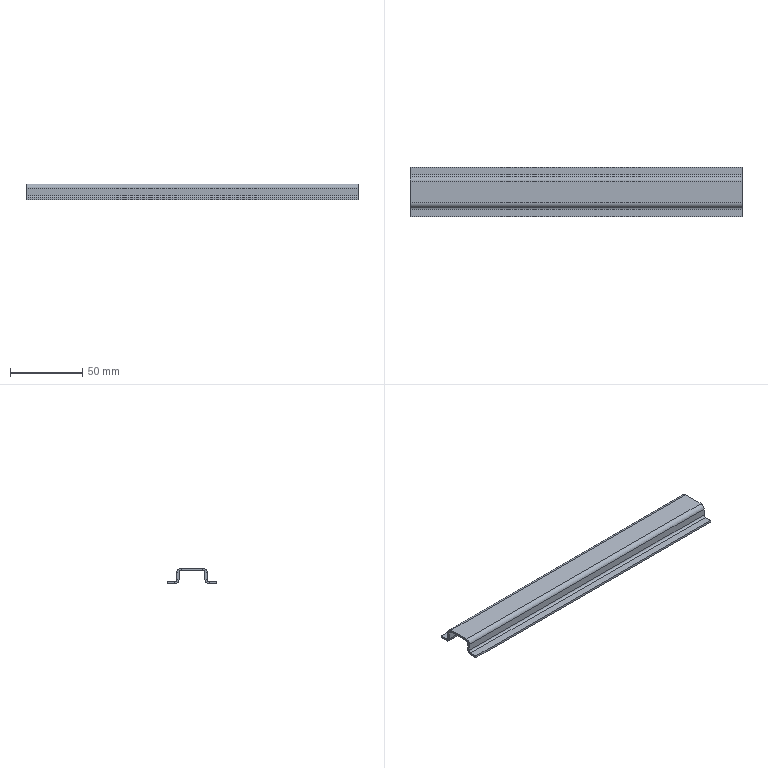Part | SolidWorks | features EdgeFlange 2, FlatPattern 1, SMBaseFlange 1, SheetMetal 1 | 1 solid | 38 faces | box 230 x 34 x 11 mm | volume 16952 mm3 | plane 30 | cylinder 8 | commonest cylinder face diameters 3 x4 6 x4
STEP:
#1=CARTESIAN_POINT('',(115.,-7.5,0.));
#2=VERTEX_POINT('',#1);
#3=CARTESIAN_POINT('',(115.,7.5,0.));
#4=VERTEX_POINT('',#3);
#5=CARTESIAN_POINT('',(115.,-7.5,0.));
#6=DIRECTION('',(0.,1.,0.));
#7=VECTOR('',#6,1000.);
#8=LINE('',#5,#7);
#9=EDGE_CURVE('',#2,#4,#8,.T.);
#10=ORIENTED_EDGE('',*,*,#9,.F.);
#11=CARTESIAN_POINT('',(115.,-7.5,-1.5));
#12=VERTEX_POINT('',#11);
#13=CARTESIAN_POINT('',(115.,-7.5,-1.5));
#14=DIRECTION('',(0.,0.,1.));
#15=VECTOR('',#14,1000.);
#16=LINE('',#13,#15);
#17=EDGE_CURVE('',#12,#2,#16,.T.);
#18=ORIENTED_EDGE('',*,*,#17,.F.);
#19=CARTESIAN_POINT('',(115.,7.5,-1.5));
#20=VERTEX_POINT('',#19);
#21=CARTESIAN_POINT('',(115.,-7.5,-1.5));
#22=DIRECTION('',(0.,1.,0.));
#23=VECTOR('',#22,1000.);
#24=LINE('',#21,#23);
#25=EDGE_CURVE('',#12,#20,#24,.T.);
#26=ORIENTED_EDGE('',*,*,#25,.T.);
#27=CARTESIAN_POINT('',(115.,7.5,-1.5));
#28=DIRECTION('',(0.,0.,1.));
#29=VECTOR('',#28,1000.);
#30=LINE('',#27,#29);
#31=EDGE_CURVE('',#20,#4,#30,.T.);
#32=ORIENTED_EDGE('',*,*,#31,.T.);
#33=EDGE_LOOP('',(#10,#18,#26,#32));
#34=FACE_OUTER_BOUND('',#33,.T.);
#35=CARTESIAN_POINT('',(115.,-7.5,-1.5));
#36=DIRECTION('',(1.,0.,0.));
#37=DIRECTION('',(0.,0.,-1.));
#38=AXIS2_PLACEMENT_3D('',#35,#36,#37);
#39=PLANE('',#38);
#40=ADVANCED_FACE('',(#34),#39,.T.);
#41=CARTESIAN_POINT('',(-115.,7.5,0.));
#42=VERTEX_POINT('',#41);
#43=CARTESIAN_POINT('',(-115.,-7.5,0.));
#44=VERTEX_POINT('',#43);
#45=CARTESIAN_POINT('',(-115.,-7.5,0.));
#46=DIRECTION('',(0.,-1.,0.));
#47=VECTOR('',#46,1000.);
#48=LINE('',#45,#47);
#49=EDGE_CURVE('',#42,#44,#48,.T.);
#50=ORIENTED_EDGE('',*,*,#49,.F.);
#51=CARTESIAN_POINT('',(-115.,7.5,-1.5));
#52=VERTEX_POINT('',#51);
#53=CARTESIAN_POINT('',(-115.,7.5,-1.5));
#54=DIRECTION('',(0.,0.,1.));
#55=VECTOR('',#54,1000.);
#56=LINE('',#53,#55);
#57=EDGE_CURVE('',#52,#42,#56,.T.);
#58=ORIENTED_EDGE('',*,*,#57,.F.);
#59=CARTESIAN_POINT('',(-115.,-7.5,-1.5));
#60=VERTEX_POINT('',#59);
#61=CARTESIAN_POINT('',(-115.,-7.5,-1.5));
#62=DIRECTION('',(0.,-1.,0.));
#63=VECTOR('',#62,1000.);
#64=LINE('',#61,#63);
#65=EDGE_CURVE('',#52,#60,#64,.T.);
#66=ORIENTED_EDGE('',*,*,#65,.T.);
#67=CARTESIAN_POINT('',(-115.,-7.5,-1.5));
#68=DIRECTION('',(0.,0.,1.));
#69=VECTOR('',#68,1000.);
#70=LINE('',#67,#69);
#71=EDGE_CURVE('',#60,#44,#70,.T.);
#72=ORIENTED_EDGE('',*,*,#71,.T.);
#73=EDGE_LOOP('',(#50,#58,#66,#72));
#74=FACE_OUTER_BOUND('',#73,.T.);
#75=CARTESIAN_POINT('',(-115.,-7.5,-1.5));
#76=DIRECTION('',(-1.,0.,0.));
#77=DIRECTION('',(0.,0.,1.));
#78=AXIS2_PLACEMENT_3D('',#75,#76,#77);
#79=PLANE('',#78);
#80=ADVANCED_FACE('',(#74),#79,.T.);
#81=ORIENTED_EDGE('',*,*,#25,.F.);
#82=CARTESIAN_POINT('',(-115.,-7.5,-1.5));
#83=DIRECTION('',(1.,0.,0.));
#84=VECTOR('',#83,1000.);
#85=LINE('',#82,#84);
#86=EDGE_CURVE('',#60,#12,#85,.T.);
#87=ORIENTED_EDGE('',*,*,#86,.F.);
#88=ORIENTED_EDGE('',*,*,#65,.F.);
#89=CARTESIAN_POINT('',(-115.,7.5,-1.5));
#90=DIRECTION('',(-1.,0.,0.));
#91=VECTOR('',#90,1000.);
#92=LINE('',#89,#91);
#93=EDGE_CURVE('',#20,#52,#92,.T.);
#94=ORIENTED_EDGE('',*,*,#93,.F.);
#95=EDGE_LOOP('',(#81,#87,#88,#94));
#96=FACE_OUTER_BOUND('',#95,.T.);
#97=CARTESIAN_POINT('',(0.,0.,-1.5));
#98=DIRECTION('',(0.,0.,-1.));
#99=DIRECTION('',(-1.,0.,0.));
#100=AXIS2_PLACEMENT_3D('',#97,#98,#99);
#101=PLANE('',#100);
#102=ADVANCED_FACE('',(#96),#101,.T.);
#103=ORIENTED_EDGE('',*,*,#9,.T.);
#104=CARTESIAN_POINT('',(-115.,7.5,0.));
#105=DIRECTION('',(-1.,0.,0.));
#106=VECTOR('',#105,1000.);
#107=LINE('',#104,#106);
#108=EDGE_CURVE('',#4,#42,#107,.T.);
#109=ORIENTED_EDGE('',*,*,#108,.T.);
#110=ORIENTED_EDGE('',*,*,#49,.T.);
#111=CARTESIAN_POINT('',(-115.,-7.5,0.));
#112=DIRECTION('',(1.,0.,0.));
#113=VECTOR('',#112,1000.);
#114=LINE('',#111,#113);
#115=EDGE_CURVE('',#44,#2,#114,.T.);
#116=ORIENTED_EDGE('',*,*,#115,.T.);
#117=EDGE_LOOP('',(#103,#109,#110,#116));
#118=FACE_OUTER_BOUND('',#117,.T.);
#119=CARTESIAN_POINT('',(0.,0.,0.));
#120=DIRECTION('',(0.,0.,-1.));
#121=DIRECTION('',(-1.,0.,0.));
#122=AXIS2_PLACEMENT_3D('',#119,#120,#121);
#123=PLANE('',#122);
#124=ADVANCED_FACE('',(#118),#123,.F.);
#125=CARTESIAN_POINT('',(-115.,9.,-3.));
#126=VERTEX_POINT('',#125);
#127=CARTESIAN_POINT('',(-115.,10.5,-3.));
#128=VERTEX_POINT('',#127);
#129=CARTESIAN_POINT('',(-115.,10.5,-3.));
#130=DIRECTION('',(0.,1.,0.));
#131=VECTOR('',#130,1000.);
#132=LINE('',#129,#131);
#133=EDGE_CURVE('',#126,#128,#132,.T.);
#134=ORIENTED_EDGE('',*,*,#133,.F.);
#135=CARTESIAN_POINT('',(-115.,7.5,-3.));
#136=DIRECTION('',(-1.,0.,0.));
#137=DIRECTION('',(0.,0.,-1.));
#138=AXIS2_PLACEMENT_3D('',#135,#136,#137);
#139=CIRCLE('',#138,1.5);
#140=EDGE_CURVE('',#52,#126,#139,.T.);
#141=ORIENTED_EDGE('',*,*,#140,.F.);
#142=ORIENTED_EDGE('',*,*,#57,.T.);
#143=CARTESIAN_POINT('',(-115.,7.5,-3.));
#144=DIRECTION('',(-1.,0.,0.));
#145=DIRECTION('',(0.,0.,-1.));
#146=AXIS2_PLACEMENT_3D('',#143,#144,#145);
#147=CIRCLE('',#146,3.);
#148=EDGE_CURVE('',#42,#128,#147,.T.);
#149=ORIENTED_EDGE('',*,*,#148,.T.);
#150=EDGE_LOOP('',(#134,#141,#142,#149));
#151=FACE_OUTER_BOUND('',#150,.T.);
#152=CARTESIAN_POINT('',(-115.,7.5,-3.));
#153=DIRECTION('',(-1.,0.,0.));
#154=DIRECTION('',(0.,0.,1.));
#155=AXIS2_PLACEMENT_3D('',#152,#153,#154);
#156=PLANE('',#155);
#157=ADVANCED_FACE('',(#151),#156,.T.);
#158=CARTESIAN_POINT('',(115.,9.,-3.));
#159=VERTEX_POINT('',#158);
#160=CARTESIAN_POINT('',(115.,7.5,-3.));
#161=DIRECTION('',(1.,0.,0.));
#162=DIRECTION('',(0.,0.,-1.));
#163=AXIS2_PLACEMENT_3D('',#160,#161,#162);
#164=CIRCLE('',#163,1.5);
#165=EDGE_CURVE('',#159,#20,#164,.T.);
#166=ORIENTED_EDGE('',*,*,#165,.F.);
#167=CARTESIAN_POINT('',(115.,10.5,-3.));
#168=VERTEX_POINT('',#167);
#169=CARTESIAN_POINT('',(115.,9.,-3.));
#170=DIRECTION('',(0.,1.,0.));
#171=VECTOR('',#170,1000.);
#172=LINE('',#169,#171);
#173=EDGE_CURVE('',#159,#168,#172,.T.);
#174=ORIENTED_EDGE('',*,*,#173,.T.);
#175=CARTESIAN_POINT('',(115.,7.5,-3.));
#176=DIRECTION('',(1.,0.,0.));
#177=DIRECTION('',(0.,0.,-1.));
#178=AXIS2_PLACEMENT_3D('',#175,#176,#177);
#179=CIRCLE('',#178,3.);
#180=EDGE_CURVE('',#168,#4,#179,.T.);
#181=ORIENTED_EDGE('',*,*,#180,.T.);
#182=ORIENTED_EDGE('',*,*,#31,.F.);
#183=EDGE_LOOP('',(#166,#174,#181,#182));
#184=FACE_OUTER_BOUND('',#183,.T.);
#185=CARTESIAN_POINT('',(115.,7.5,-3.));
#186=DIRECTION('',(-1.,0.,0.));
#187=DIRECTION('',(0.,0.,1.));
#188=AXIS2_PLACEMENT_3D('',#185,#186,#187);
#189=PLANE('',#188);
#190=ADVANCED_FACE('',(#184),#189,.F.);
#191=ORIENTED_EDGE('',*,*,#108,.F.);
#192=ORIENTED_EDGE('',*,*,#180,.F.);
#193=CARTESIAN_POINT('',(-115.,10.5,-3.));
#194=DIRECTION('',(-1.,0.,0.));
#195=VECTOR('',#194,1000.);
#196=LINE('',#193,#195);
#197=EDGE_CURVE('',#168,#128,#196,.T.);
#198=ORIENTED_EDGE('',*,*,#197,.T.);
#199=ORIENTED_EDGE('',*,*,#148,.F.);
#200=EDGE_LOOP('',(#191,#192,#198,#199));
#201=FACE_OUTER_BOUND('',#200,.T.);
#202=CARTESIAN_POINT('',(115.,7.5,-3.));
#203=DIRECTION('',(1.,0.,0.));
#204=DIRECTION('',(0.,1.,0.));
#205=AXIS2_PLACEMENT_3D('',#202,#203,#204);
#206=CYLINDRICAL_SURFACE('',#205,3.);
#207=ADVANCED_FACE('',(#201),#206,.T.);
#208=ORIENTED_EDGE('',*,*,#93,.T.);
#209=ORIENTED_EDGE('',*,*,#140,.T.);
#210=CARTESIAN_POINT('',(-115.,9.,-3.));
#211=DIRECTION('',(1.,0.,0.));
#212=VECTOR('',#211,1000.);
#213=LINE('',#210,#212);
#214=EDGE_CURVE('',#126,#159,#213,.T.);
#215=ORIENTED_EDGE('',*,*,#214,.T.);
#216=ORIENTED_EDGE('',*,*,#165,.T.);
#217=EDGE_LOOP('',(#208,#209,#215,#216));
#218=FACE_OUTER_BOUND('',#217,.T.);
#219=CARTESIAN_POINT('',(115.,7.5,-3.));
#220=DIRECTION('',(1.,0.,0.));
#221=DIRECTION('',(0.,1.,0.));
#222=AXIS2_PLACEMENT_3D('',#219,#220,#221);
#223=CYLINDRICAL_SURFACE('',#222,1.5);
#224=ADVANCED_FACE('',(#218),#223,.F.);
#225=ORIENTED_EDGE('',*,*,#173,.F.);
#226=CARTESIAN_POINT('',(115.,9.,-8.));
#227=VERTEX_POINT('',#226);
#228=CARTESIAN_POINT('',(115.,9.,-8.));
#229=DIRECTION('',(0.,0.,-1.));
#230=VECTOR('',#229,1000.);
#231=LINE('',#228,#230);
#232=EDGE_CURVE('',#159,#227,#231,.T.);
#233=ORIENTED_EDGE('',*,*,#232,.T.);
#234=CARTESIAN_POINT('',(115.,10.5,-8.));
#235=VERTEX_POINT('',#234);
#236=CARTESIAN_POINT('',(115.,10.5,-8.));
#237=DIRECTION('',(0.,-1.,0.));
#238=VECTOR('',#237,1000.);
#239=LINE('',#236,#238);
#240=EDGE_CURVE('',#235,#227,#239,.T.);
#241=ORIENTED_EDGE('',*,*,#240,.F.);
#242=CARTESIAN_POINT('',(115.,10.5,0.));
#243=DIRECTION('',(0.,0.,-1.));
#244=VECTOR('',#243,1000.);
#245=LINE('',#242,#244);
#246=EDGE_CURVE('',#168,#235,#245,.T.);
#247=ORIENTED_EDGE('',*,*,#246,.F.);
#248=EDGE_LOOP('',(#225,#233,#241,#247));
#249=FACE_OUTER_BOUND('',#248,.T.);
#250=CARTESIAN_POINT('',(115.,10.5,-8.));
#251=DIRECTION('',(-1.,0.,0.));
#252=DIRECTION('',(0.,0.,1.));
#253=AXIS2_PLACEMENT_3D('',#250,#251,#252);
#254=PLANE('',#253);
#255=ADVANCED_FACE('',(#249),#254,.F.);
#256=ORIENTED_EDGE('',*,*,#133,.T.);
#257=CARTESIAN_POINT('',(-115.,10.5,-8.));
#258=VERTEX_POINT('',#257);
#259=CARTESIAN_POINT('',(-115.,10.5,0.));
#260=DIRECTION('',(0.,0.,1.));
#261=VECTOR('',#260,1000.);
#262=LINE('',#259,#261);
#263=EDGE_CURVE('',#258,#128,#262,.T.);
#264=ORIENTED_EDGE('',*,*,#263,.F.);
#265=CARTESIAN_POINT('',(-115.,9.,-8.));
#266=VERTEX_POINT('',#265);
#267=CARTESIAN_POINT('',(-115.,10.5,-8.));
#268=DIRECTION('',(0.,-1.,0.));
#269=VECTOR('',#268,1000.);
#270=LINE('',#267,#269);
#271=EDGE_CURVE('',#258,#266,#270,.T.);
#272=ORIENTED_EDGE('',*,*,#271,.T.);
#273=CARTESIAN_POINT('',(-115.,9.,-1.5));
#274=DIRECTION('',(0.,0.,1.));
#275=VECTOR('',#274,1000.);
#276=LINE('',#273,#275);
#277=EDGE_CURVE('',#266,#126,#276,.T.);
#278=ORIENTED_EDGE('',*,*,#277,.T.);
#279=EDGE_LOOP('',(#256,#264,#272,#278));
#280=FACE_OUTER_BOUND('',#279,.T.);
#281=CARTESIAN_POINT('',(-115.,10.5,-1.5));
#282=DIRECTION('',(1.,0.,0.));
#283=DIRECTION('',(0.,0.,-1.));
#284=AXIS2_PLACEMENT_3D('',#281,#282,#283);
#285=PLANE('',#284);
#286=ADVANCED_FACE('',(#280),#285,.F.);
#287=ORIENTED_EDGE('',*,*,#197,.F.);
#288=ORIENTED_EDGE('',*,*,#246,.T.);
#289=CARTESIAN_POINT('',(0.,10.5,-8.));
#290=DIRECTION('',(-1.,0.,0.));
#291=VECTOR('',#290,1000.);
#292=LINE('',#289,#291);
#293=EDGE_CURVE('',#235,#258,#292,.T.);
#294=ORIENTED_EDGE('',*,*,#293,.T.);
#295=ORIENTED_EDGE('',*,*,#263,.T.);
#296=EDGE_LOOP('',(#287,#288,#294,#295));
#297=FACE_OUTER_BOUND('',#296,.T.);
#298=CARTESIAN_POINT('',(0.,10.5,0.));
#299=DIRECTION('',(0.,-1.,0.));
#300=DIRECTION('',(0.,0.,-1.));
#301=AXIS2_PLACEMENT_3D('',#298,#299,#300);
#302=PLANE('',#301);
#303=ADVANCED_FACE('',(#297),#302,.F.);
#304=ORIENTED_EDGE('',*,*,#232,.F.);
#305=ORIENTED_EDGE('',*,*,#214,.F.);
#306=ORIENTED_EDGE('',*,*,#277,.F.);
#307=CARTESIAN_POINT('',(-115.,9.,-8.));
#308=DIRECTION('',(-1.,0.,0.));
#309=VECTOR('',#308,1000.);
#310=LINE('',#307,#309);
#311=EDGE_CURVE('',#227,#266,#310,.T.);
#312=ORIENTED_EDGE('',*,*,#311,.F.);
#313=EDGE_LOOP('',(#304,#305,#306,#312));
#314=FACE_OUTER_BOUND('',#313,.T.);
#315=CARTESIAN_POINT('',(0.,9.,0.));
#316=DIRECTION('',(0.,-1.,0.));
#317=DIRECTION('',(0.,0.,-1.));
#318=AXIS2_PLACEMENT_3D('',#315,#316,#317);
#319=PLANE('',#318);
#320=ADVANCED_FACE('',(#314),#319,.T.);
#321=CARTESIAN_POINT('',(115.,-9.,-3.));
#322=VERTEX_POINT('',#321);
#323=CARTESIAN_POINT('',(115.,-10.5,-3.));
#324=VERTEX_POINT('',#323);
#325=CARTESIAN_POINT('',(115.,-10.5,-3.));
#326=DIRECTION('',(0.,-1.,0.));
#327=VECTOR('',#326,1000.);
#328=LINE('',#325,#327);
#329=EDGE_CURVE('',#322,#324,#328,.T.);
#330=ORIENTED_EDGE('',*,*,#329,.F.);
#331=CARTESIAN_POINT('',(115.,-7.5,-3.));
#332=DIRECTION('',(1.,0.,0.));
#333=DIRECTION('',(0.,0.,1.));
#334=AXIS2_PLACEMENT_3D('',#331,#332,#333);
#335=CIRCLE('',#334,1.5);
#336=EDGE_CURVE('',#12,#322,#335,.T.);
#337=ORIENTED_EDGE('',*,*,#336,.F.);
#338=ORIENTED_EDGE('',*,*,#17,.T.);
#339=CARTESIAN_POINT('',(115.,-7.5,-3.));
#340=DIRECTION('',(1.,0.,0.));
#341=DIRECTION('',(0.,0.,1.));
#342=AXIS2_PLACEMENT_3D('',#339,#340,#341);
#343=CIRCLE('',#342,3.);
#344=EDGE_CURVE('',#2,#324,#343,.T.);
#345=ORIENTED_EDGE('',*,*,#344,.T.);
#346=EDGE_LOOP('',(#330,#337,#338,#345));
#347=FACE_OUTER_BOUND('',#346,.T.);
#348=CARTESIAN_POINT('',(115.,-7.5,-3.));
#349=DIRECTION('',(1.,0.,0.));
#350=DIRECTION('',(0.,0.,-1.));
#351=AXIS2_PLACEMENT_3D('',#348,#349,#350);
#352=PLANE('',#351);
#353=ADVANCED_FACE('',(#347),#352,.T.);
#354=CARTESIAN_POINT('',(-115.,-9.,-3.));
#355=VERTEX_POINT('',#354);
#356=CARTESIAN_POINT('',(-115.,-7.5,-3.));
#357=DIRECTION('',(-1.,0.,0.));
#358=DIRECTION('',(0.,0.,1.));
#359=AXIS2_PLACEMENT_3D('',#356,#357,#358);
#360=CIRCLE('',#359,1.5);
#361=EDGE_CURVE('',#355,#60,#360,.T.);
#362=ORIENTED_EDGE('',*,*,#361,.F.);
#363=CARTESIAN_POINT('',(-115.,-10.5,-3.));
#364=VERTEX_POINT('',#363);
#365=CARTESIAN_POINT('',(-115.,-9.,-3.));
#366=DIRECTION('',(0.,-1.,0.));
#367=VECTOR('',#366,1000.);
#368=LINE('',#365,#367);
#369=EDGE_CURVE('',#355,#364,#368,.T.);
#370=ORIENTED_EDGE('',*,*,#369,.T.);
#371=CARTESIAN_POINT('',(-115.,-7.5,-3.));
#372=DIRECTION('',(-1.,0.,0.));
#373=DIRECTION('',(0.,0.,1.));
#374=AXIS2_PLACEMENT_3D('',#371,#372,#373);
#375=CIRCLE('',#374,3.);
#376=EDGE_CURVE('',#364,#44,#375,.T.);
#377=ORIENTED_EDGE('',*,*,#376,.T.);
#378=ORIENTED_EDGE('',*,*,#71,.F.);
#379=EDGE_LOOP('',(#362,#370,#377,#378));
#380=FACE_OUTER_BOUND('',#379,.T.);
#381=CARTESIAN_POINT('',(-115.,-7.5,-3.));
#382=DIRECTION('',(1.,0.,0.));
#383=DIRECTION('',(0.,0.,-1.));
#384=AXIS2_PLACEMENT_3D('',#381,#382,#383);
#385=PLANE('',#384);
#386=ADVANCED_FACE('',(#380),#385,.F.);
#387=ORIENTED_EDGE('',*,*,#115,.F.);
#388=ORIENTED_EDGE('',*,*,#376,.F.);
#389=CARTESIAN_POINT('',(115.,-10.5,-3.));
#390=DIRECTION('',(1.,0.,0.));
#391=VECTOR('',#390,1000.);
#392=LINE('',#389,#391);
#393=EDGE_CURVE('',#364,#324,#392,.T.);
#394=ORIENTED_EDGE('',*,*,#393,.T.);
#395=ORIENTED_EDGE('',*,*,#344,.F.);
#396=EDGE_LOOP('',(#387,#388,#394,#395));
#397=FACE_OUTER_BOUND('',#396,.T.);
#398=CARTESIAN_POINT('',(-115.,-7.5,-3.));
#399=DIRECTION('',(-1.,0.,0.));
#400=DIRECTION('',(0.,-1.,0.));
#401=AXIS2_PLACEMENT_3D('',#398,#399,#400);
#402=CYLINDRICAL_SURFACE('',#401,3.);
#403=ADVANCED_FACE('',(#397),#402,.T.);
#404=ORIENTED_EDGE('',*,*,#86,.T.);
#405=ORIENTED_EDGE('',*,*,#336,.T.);
#406=CARTESIAN_POINT('',(115.,-9.,-3.));
#407=DIRECTION('',(-1.,0.,0.));
#408=VECTOR('',#407,1000.);
#409=LINE('',#406,#408);
#410=EDGE_CURVE('',#322,#355,#409,.T.);
#411=ORIENTED_EDGE('',*,*,#410,.T.);
#412=ORIENTED_EDGE('',*,*,#361,.T.);
#413=EDGE_LOOP('',(#404,#405,#411,#412));
#414=FACE_OUTER_BOUND('',#413,.T.);
#415=CARTESIAN_POINT('',(-115.,-7.5,-3.));
#416=DIRECTION('',(-1.,0.,0.));
#417=DIRECTION('',(0.,-1.,0.));
#418=AXIS2_PLACEMENT_3D('',#415,#416,#417);
#419=CYLINDRICAL_SURFACE('',#418,1.5);
#420=ADVANCED_FACE('',(#414),#419,.F.);
#421=ORIENTED_EDGE('',*,*,#369,.F.);
#422=CARTESIAN_POINT('',(-115.,-9.,-8.));
#423=VERTEX_POINT('',#422);
#424=CARTESIAN_POINT('',(-115.,-9.,-8.));
#425=DIRECTION('',(0.,0.,-1.));
#426=VECTOR('',#425,1000.);
#427=LINE('',#424,#426);
#428=EDGE_CURVE('',#355,#423,#427,.T.);
#429=ORIENTED_EDGE('',*,*,#428,.T.);
#430=CARTESIAN_POINT('',(-115.,-10.5,-8.));
#431=VERTEX_POINT('',#430);
#432=CARTESIAN_POINT('',(-115.,-10.5,-8.));
#433=DIRECTION('',(0.,1.,0.));
#434=VECTOR('',#433,1000.);
#435=LINE('',#432,#434);
#436=EDGE_CURVE('',#431,#423,#435,.T.);
#437=ORIENTED_EDGE('',*,*,#436,.F.);
#438=CARTESIAN_POINT('',(-115.,-10.5,0.));
#439=DIRECTION('',(0.,0.,-1.));
#440=VECTOR('',#439,1000.);
#441=LINE('',#438,#440);
#442=EDGE_CURVE('',#364,#431,#441,.T.);
#443=ORIENTED_EDGE('',*,*,#442,.F.);
#444=EDGE_LOOP('',(#421,#429,#437,#443));
#445=FACE_OUTER_BOUND('',#444,.T.);
#446=CARTESIAN_POINT('',(-115.,-10.5,-8.));
#447=DIRECTION('',(1.,0.,0.));
#448=DIRECTION('',(0.,0.,-1.));
#449=AXIS2_PLACEMENT_3D('',#446,#447,#448);
#450=PLANE('',#449);
#451=ADVANCED_FACE('',(#445),#450,.F.);
#452=ORIENTED_EDGE('',*,*,#329,.T.);
#453=CARTESIAN_POINT('',(115.,-10.5,-8.));
#454=VERTEX_POINT('',#453);
#455=CARTESIAN_POINT('',(115.,-10.5,0.));
#456=DIRECTION('',(0.,0.,1.));
#457=VECTOR('',#456,1000.);
#458=LINE('',#455,#457);
#459=EDGE_CURVE('',#454,#324,#458,.T.);
#460=ORIENTED_EDGE('',*,*,#459,.F.);
#461=CARTESIAN_POINT('',(115.,-9.,-8.));
#462=VERTEX_POINT('',#461);
#463=CARTESIAN_POINT('',(115.,-10.5,-8.));
#464=DIRECTION('',(0.,1.,0.));
#465=VECTOR('',#464,1000.);
#466=LINE('',#463,#465);
#467=EDGE_CURVE('',#454,#462,#466,.T.);
#468=ORIENTED_EDGE('',*,*,#467,.T.);
#469=CARTESIAN_POINT('',(115.,-9.,-1.5));
#470=DIRECTION('',(0.,0.,1.));
#471=VECTOR('',#470,1000.);
#472=LINE('',#469,#471);
#473=EDGE_CURVE('',#462,#322,#472,.T.);
#474=ORIENTED_EDGE('',*,*,#473,.T.);
#475=EDGE_LOOP('',(#452,#460,#468,#474));
#476=FACE_OUTER_BOUND('',#475,.T.);
#477=CARTESIAN_POINT('',(115.,-10.5,-1.5));
#478=DIRECTION('',(-1.,0.,0.));
#479=DIRECTION('',(0.,0.,1.));
#480=AXIS2_PLACEMENT_3D('',#477,#478,#479);
#481=PLANE('',#480);
#482=ADVANCED_FACE('',(#476),#481,.F.);
#483=ORIENTED_EDGE('',*,*,#393,.F.);
#484=ORIENTED_EDGE('',*,*,#442,.T.);
#485=CARTESIAN_POINT('',(0.,-10.5,-8.));
#486=DIRECTION('',(1.,0.,0.));
#487=VECTOR('',#486,1000.);
#488=LINE('',#485,#487);
#489=EDGE_CURVE('',#431,#454,#488,.T.);
#490=ORIENTED_EDGE('',*,*,#489,.T.);
#491=ORIENTED_EDGE('',*,*,#459,.T.);
#492=EDGE_LOOP('',(#483,#484,#490,#491));
#493=FACE_OUTER_BOUND('',#492,.T.);
#494=CARTESIAN_POINT('',(0.,-10.5,0.));
#495=DIRECTION('',(0.,1.,0.));
#496=DIRECTION('',(0.,0.,1.));
#497=AXIS2_PLACEMENT_3D('',#494,#495,#496);
#498=PLANE('',#497);
#499=ADVANCED_FACE('',(#493),#498,.F.);
#500=ORIENTED_EDGE('',*,*,#428,.F.);
#501=ORIENTED_EDGE('',*,*,#410,.F.);
#502=ORIENTED_EDGE('',*,*,#473,.F.);
#503=CARTESIAN_POINT('',(115.,-9.,-8.));
#504=DIRECTION('',(1.,0.,0.));
#505=VECTOR('',#504,1000.);
#506=LINE('',#503,#505);
#507=EDGE_CURVE('',#423,#462,#506,.T.);
#508=ORIENTED_EDGE('',*,*,#507,.F.);
#509=EDGE_LOOP('',(#500,#501,#502,#508));
#510=FACE_OUTER_BOUND('',#509,.T.);
#511=CARTESIAN_POINT('',(0.,-9.,0.));
#512=DIRECTION('',(0.,1.,0.));
#513=DIRECTION('',(0.,0.,1.));
#514=AXIS2_PLACEMENT_3D('',#511,#512,#513);
#515=PLANE('',#514);
#516=ADVANCED_FACE('',(#510),#515,.T.);
#517=CARTESIAN_POINT('',(115.,12.,-9.5));
#518=VERTEX_POINT('',#517);
#519=CARTESIAN_POINT('',(115.,12.,-11.));
#520=VERTEX_POINT('',#519);
#521=CARTESIAN_POINT('',(115.,12.,-11.));
#522=DIRECTION('',(0.,0.,-1.));
#523=VECTOR('',#522,1000.);
#524=LINE('',#521,#523);
#525=EDGE_CURVE('',#518,#520,#524,.T.);
#526=ORIENTED_EDGE('',*,*,#525,.F.);
#527=CARTESIAN_POINT('',(115.,12.,-8.));
#528=DIRECTION('',(1.,0.,0.));
#529=DIRECTION('',(0.,0.,1.));
#530=AXIS2_PLACEMENT_3D('',#527,#528,#529);
#531=CIRCLE('',#530,1.5);
#532=EDGE_CURVE('',#235,#518,#531,.T.);
#533=ORIENTED_EDGE('',*,*,#532,.F.);
#534=ORIENTED_EDGE('',*,*,#240,.T.);
#535=CARTESIAN_POINT('',(115.,12.,-8.));
#536=DIRECTION('',(1.,0.,0.));
#537=DIRECTION('',(0.,0.,1.));
#538=AXIS2_PLACEMENT_3D('',#535,#536,#537);
#539=CIRCLE('',#538,3.);
#540=EDGE_CURVE('',#227,#520,#539,.T.);
#541=ORIENTED_EDGE('',*,*,#540,.T.);
#542=EDGE_LOOP('',(#526,#533,#534,#541));
#543=FACE_OUTER_BOUND('',#542,.T.);
#544=CARTESIAN_POINT('',(115.,12.,-8.));
#545=DIRECTION('',(1.,0.,0.));
#546=DIRECTION('',(0.,0.,-1.));
#547=AXIS2_PLACEMENT_3D('',#544,#545,#546);
#548=PLANE('',#547);
#549=ADVANCED_FACE('',(#543),#548,.T.);
#550=CARTESIAN_POINT('',(-115.,12.,-9.5));
#551=VERTEX_POINT('',#550);
#552=CARTESIAN_POINT('',(-115.,12.,-8.));
#553=DIRECTION('',(-1.,0.,0.));
#554=DIRECTION('',(0.,0.,1.));
#555=AXIS2_PLACEMENT_3D('',#552,#553,#554);
#556=CIRCLE('',#555,1.5);
#557=EDGE_CURVE('',#551,#258,#556,.T.);
#558=ORIENTED_EDGE('',*,*,#557,.F.);
#559=CARTESIAN_POINT('',(-115.,12.,-11.));
#560=VERTEX_POINT('',#559);
#561=CARTESIAN_POINT('',(-115.,12.,-9.5));
#562=DIRECTION('',(0.,0.,-1.));
#563=VECTOR('',#562,1000.);
#564=LINE('',#561,#563);
#565=EDGE_CURVE('',#551,#560,#564,.T.);
#566=ORIENTED_EDGE('',*,*,#565,.T.);
#567=CARTESIAN_POINT('',(-115.,12.,-8.));
#568=DIRECTION('',(-1.,0.,0.));
#569=DIRECTION('',(0.,0.,1.));
#570=AXIS2_PLACEMENT_3D('',#567,#568,#569);
#571=CIRCLE('',#570,3.);
#572=EDGE_CURVE('',#560,#266,#571,.T.);
#573=ORIENTED_EDGE('',*,*,#572,.T.);
#574=ORIENTED_EDGE('',*,*,#271,.F.);
#575=EDGE_LOOP('',(#558,#566,#573,#574));
#576=FACE_OUTER_BOUND('',#575,.T.);
#577=CARTESIAN_POINT('',(-115.,12.,-8.));
#578=DIRECTION('',(1.,0.,0.));
#579=DIRECTION('',(0.,0.,-1.));
#580=AXIS2_PLACEMENT_3D('',#577,#578,#579);
#581=PLANE('',#580);
#582=ADVANCED_FACE('',(#576),#581,.F.);
#583=ORIENTED_EDGE('',*,*,#311,.T.);
#584=ORIENTED_EDGE('',*,*,#572,.F.);
#585=CARTESIAN_POINT('',(0.,12.,-11.));
#586=DIRECTION('',(-1.,0.,0.));
#587=VECTOR('',#586,1000.);
#588=LINE('',#585,#587);
#589=EDGE_CURVE('',#520,#560,#588,.T.);
#590=ORIENTED_EDGE('',*,*,#589,.F.);
#591=ORIENTED_EDGE('',*,*,#540,.F.);
#592=EDGE_LOOP('',(#583,#584,#590,#591));
#593=FACE_OUTER_BOUND('',#592,.T.);
#594=CARTESIAN_POINT('',(-115.,12.,-8.));
#595=DIRECTION('',(-1.,0.,0.));
#596=DIRECTION('',(0.,0.,-1.));
#597=AXIS2_PLACEMENT_3D('',#594,#595,#596);
#598=CYLINDRICAL_SURFACE('',#597,3.);
#599=ADVANCED_FACE('',(#593),#598,.T.);
#600=ORIENTED_EDGE('',*,*,#293,.F.);
#601=ORIENTED_EDGE('',*,*,#532,.T.);
#602=CARTESIAN_POINT('',(115.,12.,-9.5));
#603=DIRECTION('',(-1.,0.,0.));
#604=VECTOR('',#603,1000.);
#605=LINE('',#602,#604);
#606=EDGE_CURVE('',#518,#551,#605,.T.);
#607=ORIENTED_EDGE('',*,*,#606,.T.);
#608=ORIENTED_EDGE('',*,*,#557,.T.);
#609=EDGE_LOOP('',(#600,#601,#607,#608));
#610=FACE_OUTER_BOUND('',#609,.T.);
#611=CARTESIAN_POINT('',(-115.,12.,-8.));
#612=DIRECTION('',(-1.,0.,0.));
#613=DIRECTION('',(0.,0.,-1.));
#614=AXIS2_PLACEMENT_3D('',#611,#612,#613);
#615=CYLINDRICAL_SURFACE('',#614,1.5);
#616=ADVANCED_FACE('',(#610),#615,.F.);
#617=CARTESIAN_POINT('',(-115.,17.,-11.));
#618=VERTEX_POINT('',#617);
#619=CARTESIAN_POINT('',(-115.,10.5,-11.));
#620=DIRECTION('',(0.,-1.,0.));
#621=VECTOR('',#620,1000.);
#622=LINE('',#619,#621);
#623=EDGE_CURVE('',#618,#560,#622,.T.);
#624=ORIENTED_EDGE('',*,*,#623,.T.);
#625=ORIENTED_EDGE('',*,*,#565,.F.);
#626=CARTESIAN_POINT('',(-115.,17.,-9.5));
#627=VERTEX_POINT('',#626);
#628=CARTESIAN_POINT('',(-115.,0.,-9.5));
#629=DIRECTION('',(0.,-1.,0.));
#630=VECTOR('',#629,1000.);
#631=LINE('',#628,#630);
#632=EDGE_CURVE('',#627,#551,#631,.T.);
#633=ORIENTED_EDGE('',*,*,#632,.F.);
#634=CARTESIAN_POINT('',(-115.,17.,-11.));
#635=DIRECTION('',(0.,0.,1.));
#636=VECTOR('',#635,1000.);
#637=LINE('',#634,#636);
#638=EDGE_CURVE('',#618,#627,#637,.T.);
#639=ORIENTED_EDGE('',*,*,#638,.F.);
#640=EDGE_LOOP('',(#624,#625,#633,#639));
#641=FACE_OUTER_BOUND('',#640,.T.);
#642=CARTESIAN_POINT('',(-115.,10.5,-11.));
#643=DIRECTION('',(-1.,0.,0.));
#644=DIRECTION('',(0.,0.,1.));
#645=AXIS2_PLACEMENT_3D('',#642,#643,#644);
#646=PLANE('',#645);
#647=ADVANCED_FACE('',(#641),#646,.T.);
#648=CARTESIAN_POINT('',(115.,17.,-9.5));
#649=VERTEX_POINT('',#648);
#650=CARTESIAN_POINT('',(115.,0.,-9.5));
#651=DIRECTION('',(0.,1.,0.));
#652=VECTOR('',#651,1000.);
#653=LINE('',#650,#652);
#654=EDGE_CURVE('',#518,#649,#653,.T.);
#655=ORIENTED_EDGE('',*,*,#654,.F.);
#656=ORIENTED_EDGE('',*,*,#525,.T.);
#657=CARTESIAN_POINT('',(115.,17.,-11.));
#658=VERTEX_POINT('',#657);
#659=CARTESIAN_POINT('',(115.,17.,-11.));
#660=DIRECTION('',(0.,1.,0.));
#661=VECTOR('',#660,1000.);
#662=LINE('',#659,#661);
#663=EDGE_CURVE('',#520,#658,#662,.T.);
#664=ORIENTED_EDGE('',*,*,#663,.T.);
#665=CARTESIAN_POINT('',(115.,17.,-11.));
#666=DIRECTION('',(0.,0.,1.));
#667=VECTOR('',#666,1000.);
#668=LINE('',#665,#667);
#669=EDGE_CURVE('',#658,#649,#668,.T.);
#670=ORIENTED_EDGE('',*,*,#669,.T.);
#671=EDGE_LOOP('',(#655,#656,#664,#670));
#672=FACE_OUTER_BOUND('',#671,.T.);
#673=CARTESIAN_POINT('',(115.,17.,-11.));
#674=DIRECTION('',(1.,0.,0.));
#675=DIRECTION('',(0.,0.,-1.));
#676=AXIS2_PLACEMENT_3D('',#673,#674,#675);
#677=PLANE('',#676);
#678=ADVANCED_FACE('',(#672),#677,.T.);
#679=ORIENTED_EDGE('',*,*,#663,.F.);
#680=ORIENTED_EDGE('',*,*,#589,.T.);
#681=ORIENTED_EDGE('',*,*,#623,.F.);
#682=CARTESIAN_POINT('',(-115.,17.,-11.));
#683=DIRECTION('',(-1.,0.,0.));
#684=VECTOR('',#683,1000.);
#685=LINE('',#682,#684);
#686=EDGE_CURVE('',#658,#618,#685,.T.);
#687=ORIENTED_EDGE('',*,*,#686,.F.);
#688=EDGE_LOOP('',(#679,#680,#681,#687));
#689=FACE_OUTER_BOUND('',#688,.T.);
#690=CARTESIAN_POINT('',(0.,0.,-11.));
#691=DIRECTION('',(0.,0.,-1.));
#692=DIRECTION('',(-1.,0.,0.));
#693=AXIS2_PLACEMENT_3D('',#690,#691,#692);
#694=PLANE('',#693);
#695=ADVANCED_FACE('',(#689),#694,.T.);
#696=ORIENTED_EDGE('',*,*,#606,.F.);
#697=ORIENTED_EDGE('',*,*,#654,.T.);
#698=CARTESIAN_POINT('',(0.,17.,-9.5));
#699=DIRECTION('',(-1.,0.,0.));
#700=VECTOR('',#699,1000.);
#701=LINE('',#698,#700);
#702=EDGE_CURVE('',#649,#627,#701,.T.);
#703=ORIENTED_EDGE('',*,*,#702,.T.);
#704=ORIENTED_EDGE('',*,*,#632,.T.);
#705=EDGE_LOOP('',(#696,#697,#703,#704));
#706=FACE_OUTER_BOUND('',#705,.T.);
#707=CARTESIAN_POINT('',(0.,0.,-9.5));
#708=DIRECTION('',(0.,0.,-1.));
#709=DIRECTION('',(-1.,0.,0.));
#710=AXIS2_PLACEMENT_3D('',#707,#708,#709);
#711=PLANE('',#710);
#712=ADVANCED_FACE('',(#706),#711,.F.);
#713=ORIENTED_EDGE('',*,*,#702,.F.);
#714=ORIENTED_EDGE('',*,*,#669,.F.);
#715=ORIENTED_EDGE('',*,*,#686,.T.);
#716=ORIENTED_EDGE('',*,*,#638,.T.);
#717=EDGE_LOOP('',(#713,#714,#715,#716));
#718=FACE_OUTER_BOUND('',#717,.T.);
#719=CARTESIAN_POINT('',(-115.,17.,-11.));
#720=DIRECTION('',(0.,1.,0.));
#721=DIRECTION('',(0.,0.,1.));
#722=AXIS2_PLACEMENT_3D('',#719,#720,#721);
#723=PLANE('',#722);
#724=ADVANCED_FACE('',(#718),#723,.T.);
#725=CARTESIAN_POINT('',(-115.,-12.,-9.5));
#726=VERTEX_POINT('',#725);
#727=CARTESIAN_POINT('',(-115.,-12.,-11.));
#728=VERTEX_POINT('',#727);
#729=CARTESIAN_POINT('',(-115.,-12.,-11.));
#730=DIRECTION('',(0.,0.,-1.));
#731=VECTOR('',#730,1000.);
#732=LINE('',#729,#731);
#733=EDGE_CURVE('',#726,#728,#732,.T.);
#734=ORIENTED_EDGE('',*,*,#733,.F.);
#735=CARTESIAN_POINT('',(-115.,-12.,-8.));
#736=DIRECTION('',(-1.,0.,0.));
#737=DIRECTION('',(0.,0.,-1.));
#738=AXIS2_PLACEMENT_3D('',#735,#736,#737);
#739=CIRCLE('',#738,1.5);
#740=EDGE_CURVE('',#431,#726,#739,.T.);
#741=ORIENTED_EDGE('',*,*,#740,.F.);
#742=ORIENTED_EDGE('',*,*,#436,.T.);
#743=CARTESIAN_POINT('',(-115.,-12.,-8.));
#744=DIRECTION('',(-1.,0.,0.));
#745=DIRECTION('',(0.,0.,-1.));
#746=AXIS2_PLACEMENT_3D('',#743,#744,#745);
#747=CIRCLE('',#746,3.);
#748=EDGE_CURVE('',#423,#728,#747,.T.);
#749=ORIENTED_EDGE('',*,*,#748,.T.);
#750=EDGE_LOOP('',(#734,#741,#742,#749));
#751=FACE_OUTER_BOUND('',#750,.T.);
#752=CARTESIAN_POINT('',(-115.,-12.,-8.));
#753=DIRECTION('',(-1.,0.,0.));
#754=DIRECTION('',(0.,0.,1.));
#755=AXIS2_PLACEMENT_3D('',#752,#753,#754);
#756=PLANE('',#755);
#757=ADVANCED_FACE('',(#751),#756,.T.);
#758=CARTESIAN_POINT('',(115.,-12.,-9.5));
#759=VERTEX_POINT('',#758);
#760=CARTESIAN_POINT('',(115.,-12.,-8.));
#761=DIRECTION('',(1.,0.,0.));
#762=DIRECTION('',(0.,0.,-1.));
#763=AXIS2_PLACEMENT_3D('',#760,#761,#762);
#764=CIRCLE('',#763,1.5);
#765=EDGE_CURVE('',#759,#454,#764,.T.);
#766=ORIENTED_EDGE('',*,*,#765,.F.);
#767=CARTESIAN_POINT('',(115.,-12.,-11.));
#768=VERTEX_POINT('',#767);
#769=CARTESIAN_POINT('',(115.,-12.,-9.5));
#770=DIRECTION('',(0.,0.,-1.));
#771=VECTOR('',#770,1000.);
#772=LINE('',#769,#771);
#773=EDGE_CURVE('',#759,#768,#772,.T.);
#774=ORIENTED_EDGE('',*,*,#773,.T.);
#775=CARTESIAN_POINT('',(115.,-12.,-8.));
#776=DIRECTION('',(1.,0.,0.));
#777=DIRECTION('',(0.,0.,-1.));
#778=AXIS2_PLACEMENT_3D('',#775,#776,#777);
#779=CIRCLE('',#778,3.);
#780=EDGE_CURVE('',#768,#462,#779,.T.);
#781=ORIENTED_EDGE('',*,*,#780,.T.);
#782=ORIENTED_EDGE('',*,*,#467,.F.);
#783=EDGE_LOOP('',(#766,#774,#781,#782));
#784=FACE_OUTER_BOUND('',#783,.T.);
#785=CARTESIAN_POINT('',(115.,-12.,-8.));
#786=DIRECTION('',(-1.,0.,0.));
#787=DIRECTION('',(0.,0.,1.));
#788=AXIS2_PLACEMENT_3D('',#785,#786,#787);
#789=PLANE('',#788);
#790=ADVANCED_FACE('',(#784),#789,.F.);
#791=ORIENTED_EDGE('',*,*,#507,.T.);
#792=ORIENTED_EDGE('',*,*,#780,.F.);
#793=CARTESIAN_POINT('',(-115.,-12.,-11.));
#794=DIRECTION('',(-1.,0.,0.));
#795=VECTOR('',#794,1000.);
#796=LINE('',#793,#795);
#797=EDGE_CURVE('',#768,#728,#796,.T.);
#798=ORIENTED_EDGE('',*,*,#797,.T.);
#799=ORIENTED_EDGE('',*,*,#748,.F.);
#800=EDGE_LOOP('',(#791,#792,#798,#799));
#801=FACE_OUTER_BOUND('',#800,.T.);
#802=CARTESIAN_POINT('',(115.,-12.,-8.));
#803=DIRECTION('',(1.,0.,0.));
#804=DIRECTION('',(0.,0.,-1.));
#805=AXIS2_PLACEMENT_3D('',#802,#803,#804);
#806=CYLINDRICAL_SURFACE('',#805,3.);
#807=ADVANCED_FACE('',(#801),#806,.T.);
#808=ORIENTED_EDGE('',*,*,#489,.F.);
#809=ORIENTED_EDGE('',*,*,#740,.T.);
#810=CARTESIAN_POINT('',(-115.,-12.,-9.5));
#811=DIRECTION('',(1.,0.,0.));
#812=VECTOR('',#811,1000.);
#813=LINE('',#810,#812);
#814=EDGE_CURVE('',#726,#759,#813,.T.);
#815=ORIENTED_EDGE('',*,*,#814,.T.);
#816=ORIENTED_EDGE('',*,*,#765,.T.);
#817=EDGE_LOOP('',(#808,#809,#815,#816));
#818=FACE_OUTER_BOUND('',#817,.T.);
#819=CARTESIAN_POINT('',(115.,-12.,-8.));
#820=DIRECTION('',(1.,0.,0.));
#821=DIRECTION('',(0.,0.,-1.));
#822=AXIS2_PLACEMENT_3D('',#819,#820,#821);
#823=CYLINDRICAL_SURFACE('',#822,1.5);
#824=ADVANCED_FACE('',(#818),#823,.F.);
#825=CARTESIAN_POINT('',(-115.,-17.,-9.5));
#826=VERTEX_POINT('',#825);
#827=CARTESIAN_POINT('',(-115.,0.,-9.5));
#828=DIRECTION('',(0.,-1.,0.));
#829=VECTOR('',#828,1000.);
#830=LINE('',#827,#829);
#831=EDGE_CURVE('',#726,#826,#830,.T.);
#832=ORIENTED_EDGE('',*,*,#831,.F.);
#833=ORIENTED_EDGE('',*,*,#733,.T.);
#834=CARTESIAN_POINT('',(-115.,-17.,-11.));
#835=VERTEX_POINT('',#834);
#836=CARTESIAN_POINT('',(-115.,-10.5,-11.));
#837=DIRECTION('',(0.,-1.,0.));
#838=VECTOR('',#837,1000.);
#839=LINE('',#836,#838);
#840=EDGE_CURVE('',#728,#835,#839,.T.);
#841=ORIENTED_EDGE('',*,*,#840,.T.);
#842=CARTESIAN_POINT('',(-115.,-17.,-11.));
#843=DIRECTION('',(0.,0.,1.));
#844=VECTOR('',#843,1000.);
#845=LINE('',#842,#844);
#846=EDGE_CURVE('',#835,#826,#845,.T.);
#847=ORIENTED_EDGE('',*,*,#846,.T.);
#848=EDGE_LOOP('',(#832,#833,#841,#847));
#849=FACE_OUTER_BOUND('',#848,.T.);
#850=CARTESIAN_POINT('',(-115.,-10.5,-11.));
#851=DIRECTION('',(-1.,0.,0.));
#852=DIRECTION('',(0.,0.,1.));
#853=AXIS2_PLACEMENT_3D('',#850,#851,#852);
#854=PLANE('',#853);
#855=ADVANCED_FACE('',(#849),#854,.T.);
#856=CARTESIAN_POINT('',(115.,-17.,-11.));
#857=VERTEX_POINT('',#856);
#858=CARTESIAN_POINT('',(115.,-17.,-11.));
#859=DIRECTION('',(0.,1.,0.));
#860=VECTOR('',#859,1000.);
#861=LINE('',#858,#860);
#862=EDGE_CURVE('',#857,#768,#861,.T.);
#863=ORIENTED_EDGE('',*,*,#862,.T.);
#864=ORIENTED_EDGE('',*,*,#773,.F.);
#865=CARTESIAN_POINT('',(115.,-17.,-9.5));
#866=VERTEX_POINT('',#865);
#867=CARTESIAN_POINT('',(115.,0.,-9.5));
#868=DIRECTION('',(0.,1.,0.));
#869=VECTOR('',#868,1000.);
#870=LINE('',#867,#869);
#871=EDGE_CURVE('',#866,#759,#870,.T.);
#872=ORIENTED_EDGE('',*,*,#871,.F.);
#873=CARTESIAN_POINT('',(115.,-17.,-11.));
#874=DIRECTION('',(0.,0.,1.));
#875=VECTOR('',#874,1000.);
#876=LINE('',#873,#875);
#877=EDGE_CURVE('',#857,#866,#876,.T.);
#878=ORIENTED_EDGE('',*,*,#877,.F.);
#879=EDGE_LOOP('',(#863,#864,#872,#878));
#880=FACE_OUTER_BOUND('',#879,.T.);
#881=CARTESIAN_POINT('',(115.,-17.,-11.));
#882=DIRECTION('',(1.,0.,0.));
#883=DIRECTION('',(0.,0.,-1.));
#884=AXIS2_PLACEMENT_3D('',#881,#882,#883);
#885=PLANE('',#884);
#886=ADVANCED_FACE('',(#880),#885,.T.);
#887=ORIENTED_EDGE('',*,*,#797,.F.);
#888=ORIENTED_EDGE('',*,*,#862,.F.);
#889=CARTESIAN_POINT('',(-115.,-17.,-11.));
#890=DIRECTION('',(1.,0.,0.));
#891=VECTOR('',#890,1000.);
#892=LINE('',#889,#891);
#893=EDGE_CURVE('',#835,#857,#892,.T.);
#894=ORIENTED_EDGE('',*,*,#893,.F.);
#895=ORIENTED_EDGE('',*,*,#840,.F.);
#896=EDGE_LOOP('',(#887,#888,#894,#895));
#897=FACE_OUTER_BOUND('',#896,.T.);
#898=CARTESIAN_POINT('',(0.,0.,-11.));
#899=DIRECTION('',(0.,0.,1.));
#900=DIRECTION('',(1.,0.,0.));
#901=AXIS2_PLACEMENT_3D('',#898,#899,#900);
#902=PLANE('',#901);
#903=ADVANCED_FACE('',(#897),#902,.F.);
#904=ORIENTED_EDGE('',*,*,#871,.T.);
#905=ORIENTED_EDGE('',*,*,#814,.F.);
#906=ORIENTED_EDGE('',*,*,#831,.T.);
#907=CARTESIAN_POINT('',(0.,-17.,-9.5));
#908=DIRECTION('',(1.,0.,0.));
#909=VECTOR('',#908,1000.);
#910=LINE('',#907,#909);
#911=EDGE_CURVE('',#826,#866,#910,.T.);
#912=ORIENTED_EDGE('',*,*,#911,.T.);
#913=EDGE_LOOP('',(#904,#905,#906,#912));
#914=FACE_OUTER_BOUND('',#913,.T.);
#915=CARTESIAN_POINT('',(0.,0.,-9.5));
#916=DIRECTION('',(0.,0.,1.));
#917=DIRECTION('',(1.,0.,0.));
#918=AXIS2_PLACEMENT_3D('',#915,#916,#917);
#919=PLANE('',#918);
#920=ADVANCED_FACE('',(#914),#919,.T.);
#921=ORIENTED_EDGE('',*,*,#911,.F.);
#922=ORIENTED_EDGE('',*,*,#846,.F.);
#923=ORIENTED_EDGE('',*,*,#893,.T.);
#924=ORIENTED_EDGE('',*,*,#877,.T.);
#925=EDGE_LOOP('',(#921,#922,#923,#924));
#926=FACE_OUTER_BOUND('',#925,.T.);
#927=CARTESIAN_POINT('',(-115.,-17.,-11.));
#928=DIRECTION('',(0.,-1.,0.));
#929=DIRECTION('',(1.,0.,0.));
#930=AXIS2_PLACEMENT_3D('',#927,#928,#929);
#931=PLANE('',#930);
#932=ADVANCED_FACE('',(#926),#931,.T.);
#933=CLOSED_SHELL('',(#40,#80,#102,#124,#157,#190,#207,#224,#255,#286,#303,#320,#353,#386,#403,#420,#451,#482,#499,#516,#549,#582,#599,#616,#647,#678,#695,#712,#724,#757,#790,#807,#824,#855,#886,#903,#920,#932));
#934=MANIFOLD_SOLID_BREP('',#933);
#935=CARTESIAN_POINT('',(0.,0.,0.));
#936=DIRECTION('',(0.,0.,1.));
#937=DIRECTION('',(1.,0.,0.));
#938=AXIS2_PLACEMENT_3D('',#935,#936,#937);
#939=(LENGTH_UNIT()NAMED_UNIT(*)SI_UNIT(.MILLI.,.METRE.));
#940=UNCERTAINTY_MEASURE_WITH_UNIT(LENGTH_MEASURE(0.00001),#939,'','');
#941=(NAMED_UNIT(*)PLANE_ANGLE_UNIT()SI_UNIT($,.RADIAN.));
#942=(NAMED_UNIT(*)SI_UNIT($,.STERADIAN.)SOLID_ANGLE_UNIT());
#943=(GEOMETRIC_REPRESENTATION_CONTEXT(3)GLOBAL_UNCERTAINTY_ASSIGNED_CONTEXT((#940))GLOBAL_UNIT_ASSIGNED_CONTEXT((#939,#941,#942))REPRESENTATION_CONTEXT('',''));
#944=ADVANCED_BREP_SHAPE_REPRESENTATION('',(#934,#938),#943);